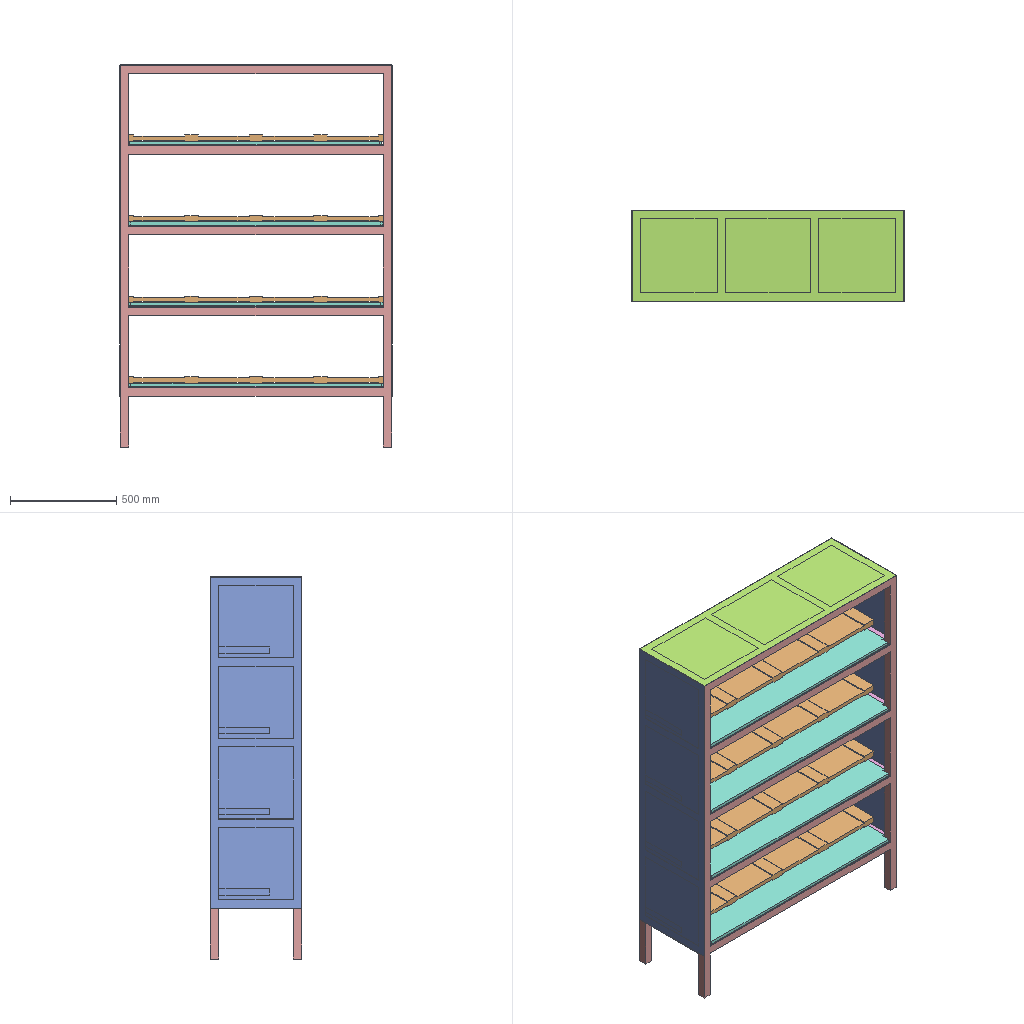Assembly | SolidWorks | 6 different items | 16 placed | box 1283 x 430 x 1802 mm
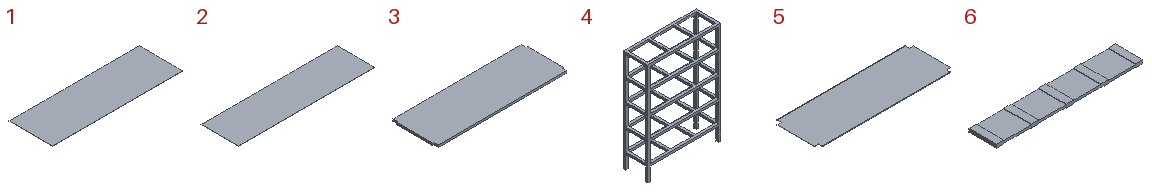Parts list (item | quantity | size | volume | features):
1 | x1 | 1280 x 430 x 1.5 mm | 825600 mm3 | features Extrusion 1
2 | x2 | 1560 x 430 x 1.5 mm | 1006200 mm3 | features Extrusion 1
3 | x4 | 1200 x 415 x 20 mm | 9928000 mm3 | features Extrusion 1, ICE 1
4 | x1 | 1280 x 430 x 1800 mm | 41920000 mm3 | features ICE 4, Extrusion 1
5 | x4 | 1280 x 430 x 6.5 mm | 834000 mm3 | features Extrusion 1, ICE 1
6 | x4 | 1280 x 240 x 30 mm | 6912000 mm3 | features Extrusion 1, ICE 1
Mates (type | each side: item.copy, entity, surface, feature):
Coincident | 4.1 face plane Boss-Extrude1 | 2.1 face plane Boss-Extrude1
Coincident | 4.1 edge | 2.1 edge | 2 times
Coincident | 4.1 face plane Boss-Extrude1 | 2.2 face plane Boss-Extrude1
Coincident | 4.1 edge | 2.2 edge | 2 times
Coincident | 4.1 face plane Boss-Extrude2 | 1.1 face plane Boss-Extrude1
Coincident | 4.1 edge | 1.1 edge
Coincident | 2.2 edge | 1.1 edge
Coincident | 4.1 face plane Boss-Extrude3 | 5.1 face plane Boss-Extrude1
Coincident | 4.1 edge | 5.1 edge | 2 times
Coincident | 4.1 face plane Boss-Extrude4 | 5.2 face plane Boss-Extrude1
Coincident | 4.1 face plane Boss-Extrude1 | 5.2 edge
Coincident | 4.1 edge | 5.2 edge
Coincident | 4.1 face plane Boss-Extrude4 | 5.3 face plane Boss-Extrude1
Coincident | 4.1 edge | 5.3 edge | 2 times
Coincident | 4.1 face plane Boss-Extrude1 | 5.4 face plane Boss-Extrude1
Coincident | 4.1 edge | 5.4 edge
Coincident | 5.1 face plane Boss-Extrude1 | 3.1 face plane Boss-Extrude1
Coincident | 4.1 face plane Boss-Extrude2 | 3.1 face plane Cut-Extrude1 | 2 times
Coincident | 5.2 face plane Boss-Extrude1 | 3.2 face plane Boss-Extrude1
Coincident | 4.1 face plane Boss-Extrude2 | 3.2 face plane Cut-Extrude1 | 2 times
Coincident | 5.3 face plane Boss-Extrude1 | 3.3 face plane Boss-Extrude1
Coincident | 4.1 face plane Boss-Extrude2 | 3.3 face plane Cut-Extrude1 | 2 times
Coincident | 2.2 face plane Boss-Extrude1 | 5.4 edge
Coincident | 5.4 face plane Boss-Extrude1 | 3.4 face plane Boss-Extrude1
Coincident | 4.1 face plane Boss-Extrude2 | 3.4 face plane Cut-Extrude1 | 2 times
Coincident | 4.1 face plane Boss-Extrude2 | 6.1 face plane Boss-Extrude1
Coincident | 3.1 face plane Boss-Extrude1 | 6.1 face plane Boss-Extrude2
Coincident | 2.1 face plane Boss-Extrude1 | 6.1 edge
Coincident | 3.2 face plane Boss-Extrude1 | 6.2 face plane Boss-Extrude2
Coincident | 4.1 face plane Boss-Extrude2 | 6.2 face plane Boss-Extrude1
Coincident | 2.2 face plane Boss-Extrude1 | 6.2 edge
Coincident | 3.3 face plane Boss-Extrude1 | 6.3 face plane Boss-Extrude2
Coincident | 4.1 face plane Boss-Extrude2 | 6.3 face plane Boss-Extrude1
Coincident | 2.2 face plane Boss-Extrude1 | 6.3 edge
Coincident | 3.4 face plane Boss-Extrude1 | 6.4 face plane Boss-Extrude2
Coincident | 4.1 face plane Boss-Extrude2 | 6.4 face plane Boss-Extrude1
Coincident | 2.2 face plane Boss-Extrude1 | 6.4 face plane Boss-Extrude2